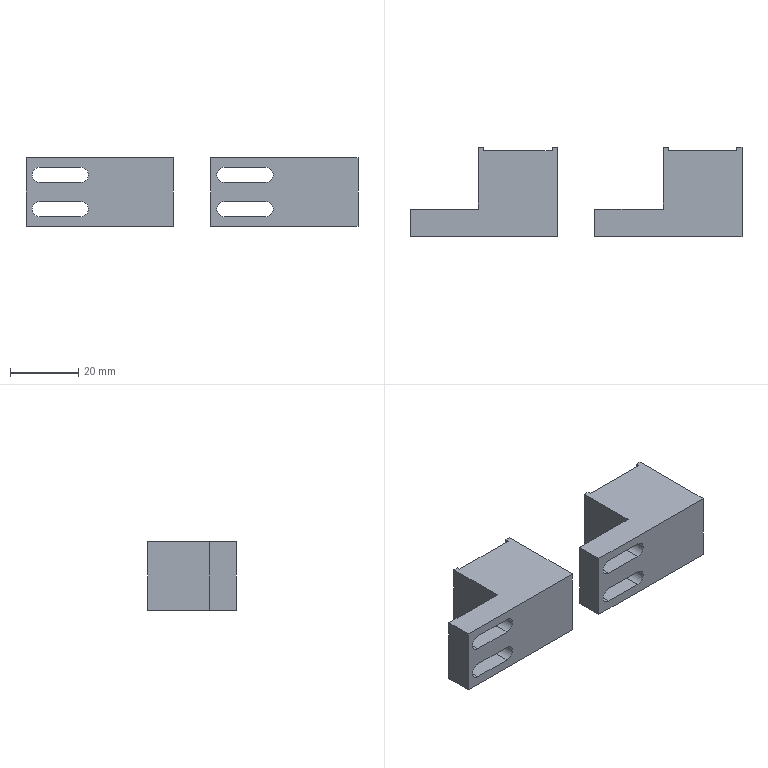Part | 2 solids | 48 faces | box 97 x 26 x 20 mm | volume 26926 mm3 | plane 32 | cylinder 12 | cone 4 | commonest cylinder face diameters 4.5 x8 3.3 x4
STEP:
#1=CARTESIAN_POINT('',(-21.5,25.,0.));
#2=VERTEX_POINT('',#1);
#3=CARTESIAN_POINT('',(-21.5,25.,20.));
#4=VERTEX_POINT('',#3);
#5=CARTESIAN_POINT('',(-21.5,25.,0.));
#6=DIRECTION('',(0.,0.,1.));
#7=VECTOR('',#6,1000.);
#8=LINE('',#5,#7);
#9=EDGE_CURVE('',#2,#4,#8,.T.);
#10=ORIENTED_EDGE('',*,*,#9,.T.);
#11=CARTESIAN_POINT('',(-1.5,25.,20.));
#12=VERTEX_POINT('',#11);
#13=CARTESIAN_POINT('',(-21.5,25.,20.));
#14=DIRECTION('',(1.,0.,0.));
#15=VECTOR('',#14,1000.);
#16=LINE('',#13,#15);
#17=EDGE_CURVE('',#4,#12,#16,.T.);
#18=ORIENTED_EDGE('',*,*,#17,.T.);
#19=CARTESIAN_POINT('',(-1.5,25.,0.));
#20=VERTEX_POINT('',#19);
#21=CARTESIAN_POINT('',(-1.5,25.,0.));
#22=DIRECTION('',(0.,0.,-1.));
#23=VECTOR('',#22,1000.);
#24=LINE('',#21,#23);
#25=EDGE_CURVE('',#12,#20,#24,.T.);
#26=ORIENTED_EDGE('',*,*,#25,.T.);
#27=CARTESIAN_POINT('',(-21.5,25.,0.));
#28=DIRECTION('',(-1.,0.,0.));
#29=VECTOR('',#28,1000.);
#30=LINE('',#27,#29);
#31=EDGE_CURVE('',#20,#2,#30,.T.);
#32=ORIENTED_EDGE('',*,*,#31,.T.);
#33=EDGE_LOOP('',(#10,#18,#26,#32));
#34=FACE_BOUND('',#33,.T.);
#35=CARTESIAN_POINT('',(-16.5,25.,11.65));
#36=VERTEX_POINT('',#35);
#37=CARTESIAN_POINT('',(-16.5,25.,10.));
#38=DIRECTION('',(0.,1.,0.));
#39=DIRECTION('',(0.,0.,1.));
#40=AXIS2_PLACEMENT_3D('',#37,#38,#39);
#41=CIRCLE('',#40,1.65);
#42=EDGE_CURVE('',#36,#36,#41,.T.);
#43=ORIENTED_EDGE('',*,*,#42,.F.);
#44=EDGE_LOOP('',(#43));
#45=FACE_BOUND('',#44,.T.);
#46=CARTESIAN_POINT('',(-6.5,25.,11.65));
#47=VERTEX_POINT('',#46);
#48=CARTESIAN_POINT('',(-6.5,25.,10.));
#49=DIRECTION('',(0.,1.,0.));
#50=DIRECTION('',(0.,0.,1.));
#51=AXIS2_PLACEMENT_3D('',#48,#49,#50);
#52=CIRCLE('',#51,1.65);
#53=EDGE_CURVE('',#47,#47,#52,.T.);
#54=ORIENTED_EDGE('',*,*,#53,.F.);
#55=EDGE_LOOP('',(#54));
#56=FACE_BOUND('',#55,.T.);
#57=CARTESIAN_POINT('',(0.,25.,0.));
#58=DIRECTION('',(0.,1.,0.));
#59=DIRECTION('',(-1.,0.,0.));
#60=AXIS2_PLACEMENT_3D('',#57,#58,#59);
#61=PLANE('',#60);
#62=ADVANCED_FACE('',(#34,#45,#56),#61,.T.);
#63=CARTESIAN_POINT('',(-1.5,26.,20.));
#64=VERTEX_POINT('',#63);
#65=CARTESIAN_POINT('',(-1.5,26.,0.));
#66=VERTEX_POINT('',#65);
#67=CARTESIAN_POINT('',(-1.5,26.,0.));
#68=DIRECTION('',(0.,0.,-1.));
#69=VECTOR('',#68,1000.);
#70=LINE('',#67,#69);
#71=EDGE_CURVE('',#64,#66,#70,.T.);
#72=ORIENTED_EDGE('',*,*,#71,.T.);
#73=CARTESIAN_POINT('',(-1.5,25.,0.));
#74=DIRECTION('',(0.,1.,0.));
#75=VECTOR('',#74,1000.);
#76=LINE('',#73,#75);
#77=EDGE_CURVE('',#20,#66,#76,.T.);
#78=ORIENTED_EDGE('',*,*,#77,.F.);
#79=ORIENTED_EDGE('',*,*,#25,.F.);
#80=CARTESIAN_POINT('',(-1.5,25.,20.));
#81=DIRECTION('',(0.,1.,0.));
#82=VECTOR('',#81,1000.);
#83=LINE('',#80,#82);
#84=EDGE_CURVE('',#12,#64,#83,.T.);
#85=ORIENTED_EDGE('',*,*,#84,.T.);
#86=EDGE_LOOP('',(#72,#78,#79,#85));
#87=FACE_BOUND('',#86,.T.);
#88=CARTESIAN_POINT('',(-1.5,25.,0.));
#89=DIRECTION('',(1.,0.,0.));
#90=DIRECTION('',(0.,0.,-1.));
#91=AXIS2_PLACEMENT_3D('',#88,#89,#90);
#92=PLANE('',#91);
#93=ADVANCED_FACE('',(#87),#92,.F.);
#94=CARTESIAN_POINT('',(-21.5,26.,0.));
#95=VERTEX_POINT('',#94);
#96=CARTESIAN_POINT('',(-21.5,26.,20.));
#97=VERTEX_POINT('',#96);
#98=CARTESIAN_POINT('',(-21.5,26.,0.));
#99=DIRECTION('',(0.,0.,1.));
#100=VECTOR('',#99,1000.);
#101=LINE('',#98,#100);
#102=EDGE_CURVE('',#95,#97,#101,.T.);
#103=ORIENTED_EDGE('',*,*,#102,.T.);
#104=CARTESIAN_POINT('',(-21.5,25.,20.));
#105=DIRECTION('',(0.,1.,0.));
#106=VECTOR('',#105,1000.);
#107=LINE('',#104,#106);
#108=EDGE_CURVE('',#4,#97,#107,.T.);
#109=ORIENTED_EDGE('',*,*,#108,.F.);
#110=ORIENTED_EDGE('',*,*,#9,.F.);
#111=CARTESIAN_POINT('',(-21.5,25.,0.));
#112=DIRECTION('',(0.,1.,0.));
#113=VECTOR('',#112,1000.);
#114=LINE('',#111,#113);
#115=EDGE_CURVE('',#2,#95,#114,.T.);
#116=ORIENTED_EDGE('',*,*,#115,.T.);
#117=EDGE_LOOP('',(#103,#109,#110,#116));
#118=FACE_BOUND('',#117,.T.);
#119=CARTESIAN_POINT('',(-21.5,25.,0.));
#120=DIRECTION('',(-1.,0.,0.));
#121=DIRECTION('',(0.,0.,1.));
#122=AXIS2_PLACEMENT_3D('',#119,#120,#121);
#123=PLANE('',#122);
#124=ADVANCED_FACE('',(#118),#123,.F.);
#125=CARTESIAN_POINT('',(-27.,0.,2.75));
#126=VERTEX_POINT('',#125);
#127=CARTESIAN_POINT('',(-27.,8.,2.75));
#128=VERTEX_POINT('',#127);
#129=CARTESIAN_POINT('',(-27.,-22.,2.75));
#130=DIRECTION('',(0.,1.,0.));
#131=VECTOR('',#130,1000.);
#132=LINE('',#129,#131);
#133=EDGE_CURVE('',#126,#128,#132,.T.);
#134=ORIENTED_EDGE('',*,*,#133,.T.);
#135=CARTESIAN_POINT('',(-39.,8.,2.75));
#136=VERTEX_POINT('',#135);
#137=CARTESIAN_POINT('',(-27.,8.,2.75));
#138=DIRECTION('',(-1.,0.,0.));
#139=VECTOR('',#138,1000.);
#140=LINE('',#137,#139);
#141=EDGE_CURVE('',#128,#136,#140,.T.);
#142=ORIENTED_EDGE('',*,*,#141,.T.);
#143=CARTESIAN_POINT('',(-39.,0.,2.75));
#144=VERTEX_POINT('',#143);
#145=CARTESIAN_POINT('',(-39.,-22.,2.75));
#146=DIRECTION('',(0.,1.,0.));
#147=VECTOR('',#146,1000.);
#148=LINE('',#145,#147);
#149=EDGE_CURVE('',#144,#136,#148,.T.);
#150=ORIENTED_EDGE('',*,*,#149,.F.);
#151=CARTESIAN_POINT('',(-43.,0.,2.75));
#152=DIRECTION('',(-1.,0.,0.));
#153=VECTOR('',#152,1000.);
#154=LINE('',#151,#153);
#155=EDGE_CURVE('',#126,#144,#154,.T.);
#156=ORIENTED_EDGE('',*,*,#155,.F.);
#157=EDGE_LOOP('',(#134,#142,#150,#156));
#158=FACE_BOUND('',#157,.T.);
#159=CARTESIAN_POINT('',(-27.,-22.,2.75));
#160=DIRECTION('',(0.,0.,-1.));
#161=DIRECTION('',(-1.,0.,0.));
#162=AXIS2_PLACEMENT_3D('',#159,#160,#161);
#163=PLANE('',#162);
#164=ADVANCED_FACE('',(#158),#163,.F.);
#165=CARTESIAN_POINT('',(-39.,0.,7.25));
#166=VERTEX_POINT('',#165);
#167=CARTESIAN_POINT('',(-39.,8.,7.25));
#168=VERTEX_POINT('',#167);
#169=CARTESIAN_POINT('',(-39.,-22.,7.25));
#170=DIRECTION('',(0.,1.,0.));
#171=VECTOR('',#170,1000.);
#172=LINE('',#169,#171);
#173=EDGE_CURVE('',#166,#168,#172,.T.);
#174=ORIENTED_EDGE('',*,*,#173,.T.);
#175=CARTESIAN_POINT('',(-27.,8.,7.25));
#176=VERTEX_POINT('',#175);
#177=CARTESIAN_POINT('',(-27.,8.,7.25));
#178=DIRECTION('',(1.,0.,0.));
#179=VECTOR('',#178,1000.);
#180=LINE('',#177,#179);
#181=EDGE_CURVE('',#168,#176,#180,.T.);
#182=ORIENTED_EDGE('',*,*,#181,.T.);
#183=CARTESIAN_POINT('',(-27.,0.,7.25));
#184=VERTEX_POINT('',#183);
#185=CARTESIAN_POINT('',(-27.,-22.,7.25));
#186=DIRECTION('',(0.,1.,0.));
#187=VECTOR('',#186,1000.);
#188=LINE('',#185,#187);
#189=EDGE_CURVE('',#184,#176,#188,.T.);
#190=ORIENTED_EDGE('',*,*,#189,.F.);
#191=CARTESIAN_POINT('',(-43.,0.,7.25));
#192=DIRECTION('',(1.,0.,0.));
#193=VECTOR('',#192,1000.);
#194=LINE('',#191,#193);
#195=EDGE_CURVE('',#166,#184,#194,.T.);
#196=ORIENTED_EDGE('',*,*,#195,.F.);
#197=EDGE_LOOP('',(#174,#182,#190,#196));
#198=FACE_BOUND('',#197,.T.);
#199=CARTESIAN_POINT('',(-27.,-22.,7.25));
#200=DIRECTION('',(0.,0.,1.));
#201=DIRECTION('',(1.,0.,0.));
#202=AXIS2_PLACEMENT_3D('',#199,#200,#201);
#203=PLANE('',#202);
#204=ADVANCED_FACE('',(#198),#203,.F.);
#205=ORIENTED_EDGE('',*,*,#189,.T.);
#206=CARTESIAN_POINT('',(-27.,8.,5.));
#207=DIRECTION('',(0.,1.,0.));
#208=DIRECTION('',(-1.,0.,0.));
#209=AXIS2_PLACEMENT_3D('',#206,#207,#208);
#210=CIRCLE('',#209,2.25);
#211=EDGE_CURVE('',#176,#128,#210,.T.);
#212=ORIENTED_EDGE('',*,*,#211,.T.);
#213=ORIENTED_EDGE('',*,*,#133,.F.);
#214=CARTESIAN_POINT('',(-27.,0.,5.));
#215=DIRECTION('',(0.,1.,0.));
#216=DIRECTION('',(0.,0.,1.));
#217=AXIS2_PLACEMENT_3D('',#214,#215,#216);
#218=CIRCLE('',#217,2.25);
#219=EDGE_CURVE('',#184,#126,#218,.T.);
#220=ORIENTED_EDGE('',*,*,#219,.F.);
#221=EDGE_LOOP('',(#205,#212,#213,#220));
#222=FACE_BOUND('',#221,.T.);
#223=CARTESIAN_POINT('',(-27.,-22.,5.));
#224=DIRECTION('',(0.,1.,0.));
#225=DIRECTION('',(-1.,0.,0.));
#226=AXIS2_PLACEMENT_3D('',#223,#224,#225);
#227=CYLINDRICAL_SURFACE('',#226,2.25);
#228=ADVANCED_FACE('',(#222),#227,.F.);
#229=CARTESIAN_POINT('',(-27.,0.,12.75));
#230=VERTEX_POINT('',#229);
#231=CARTESIAN_POINT('',(-27.,8.,12.75));
#232=VERTEX_POINT('',#231);
#233=CARTESIAN_POINT('',(-27.,-22.,12.75));
#234=DIRECTION('',(0.,1.,0.));
#235=VECTOR('',#234,1000.);
#236=LINE('',#233,#235);
#237=EDGE_CURVE('',#230,#232,#236,.T.);
#238=ORIENTED_EDGE('',*,*,#237,.T.);
#239=CARTESIAN_POINT('',(-39.,8.,12.75));
#240=VERTEX_POINT('',#239);
#241=CARTESIAN_POINT('',(-27.,8.,12.75));
#242=DIRECTION('',(-1.,0.,0.));
#243=VECTOR('',#242,1000.);
#244=LINE('',#241,#243);
#245=EDGE_CURVE('',#232,#240,#244,.T.);
#246=ORIENTED_EDGE('',*,*,#245,.T.);
#247=CARTESIAN_POINT('',(-39.,0.,12.75));
#248=VERTEX_POINT('',#247);
#249=CARTESIAN_POINT('',(-39.,-22.,12.75));
#250=DIRECTION('',(0.,1.,0.));
#251=VECTOR('',#250,1000.);
#252=LINE('',#249,#251);
#253=EDGE_CURVE('',#248,#240,#252,.T.);
#254=ORIENTED_EDGE('',*,*,#253,.F.);
#255=CARTESIAN_POINT('',(-43.,0.,12.75));
#256=DIRECTION('',(-1.,0.,0.));
#257=VECTOR('',#256,1000.);
#258=LINE('',#255,#257);
#259=EDGE_CURVE('',#230,#248,#258,.T.);
#260=ORIENTED_EDGE('',*,*,#259,.F.);
#261=EDGE_LOOP('',(#238,#246,#254,#260));
#262=FACE_BOUND('',#261,.T.);
#263=CARTESIAN_POINT('',(-27.,-22.,12.75));
#264=DIRECTION('',(0.,0.,-1.));
#265=DIRECTION('',(-1.,0.,0.));
#266=AXIS2_PLACEMENT_3D('',#263,#264,#265);
#267=PLANE('',#266);
#268=ADVANCED_FACE('',(#262),#267,.F.);
#269=CARTESIAN_POINT('',(-39.,0.,17.25));
#270=VERTEX_POINT('',#269);
#271=CARTESIAN_POINT('',(-39.,8.,17.25));
#272=VERTEX_POINT('',#271);
#273=CARTESIAN_POINT('',(-39.,-22.,17.25));
#274=DIRECTION('',(0.,1.,0.));
#275=VECTOR('',#274,1000.);
#276=LINE('',#273,#275);
#277=EDGE_CURVE('',#270,#272,#276,.T.);
#278=ORIENTED_EDGE('',*,*,#277,.T.);
#279=CARTESIAN_POINT('',(-27.,8.,17.25));
#280=VERTEX_POINT('',#279);
#281=CARTESIAN_POINT('',(-27.,8.,17.25));
#282=DIRECTION('',(1.,0.,0.));
#283=VECTOR('',#282,1000.);
#284=LINE('',#281,#283);
#285=EDGE_CURVE('',#272,#280,#284,.T.);
#286=ORIENTED_EDGE('',*,*,#285,.T.);
#287=CARTESIAN_POINT('',(-27.,0.,17.25));
#288=VERTEX_POINT('',#287);
#289=CARTESIAN_POINT('',(-27.,-22.,17.25));
#290=DIRECTION('',(0.,1.,0.));
#291=VECTOR('',#290,1000.);
#292=LINE('',#289,#291);
#293=EDGE_CURVE('',#288,#280,#292,.T.);
#294=ORIENTED_EDGE('',*,*,#293,.F.);
#295=CARTESIAN_POINT('',(-43.,0.,17.25));
#296=DIRECTION('',(1.,0.,0.));
#297=VECTOR('',#296,1000.);
#298=LINE('',#295,#297);
#299=EDGE_CURVE('',#270,#288,#298,.T.);
#300=ORIENTED_EDGE('',*,*,#299,.F.);
#301=EDGE_LOOP('',(#278,#286,#294,#300));
#302=FACE_BOUND('',#301,.T.);
#303=CARTESIAN_POINT('',(-27.,-22.,17.25));
#304=DIRECTION('',(0.,0.,1.));
#305=DIRECTION('',(1.,0.,0.));
#306=AXIS2_PLACEMENT_3D('',#303,#304,#305);
#307=PLANE('',#306);
#308=ADVANCED_FACE('',(#302),#307,.F.);
#309=ORIENTED_EDGE('',*,*,#293,.T.);
#310=CARTESIAN_POINT('',(-27.,8.,15.));
#311=DIRECTION('',(0.,1.,0.));
#312=DIRECTION('',(1.,0.,0.));
#313=AXIS2_PLACEMENT_3D('',#310,#311,#312);
#314=CIRCLE('',#313,2.25);
#315=EDGE_CURVE('',#280,#232,#314,.T.);
#316=ORIENTED_EDGE('',*,*,#315,.T.);
#317=ORIENTED_EDGE('',*,*,#237,.F.);
#318=CARTESIAN_POINT('',(-27.,0.,15.));
#319=DIRECTION('',(0.,1.,0.));
#320=DIRECTION('',(0.,0.,1.));
#321=AXIS2_PLACEMENT_3D('',#318,#319,#320);
#322=CIRCLE('',#321,2.25);
#323=EDGE_CURVE('',#288,#230,#322,.T.);
#324=ORIENTED_EDGE('',*,*,#323,.F.);
#325=EDGE_LOOP('',(#309,#316,#317,#324));
#326=FACE_BOUND('',#325,.T.);
#327=CARTESIAN_POINT('',(-27.,-22.,15.));
#328=DIRECTION('',(0.,1.,0.));
#329=DIRECTION('',(-1.,0.,0.));
#330=AXIS2_PLACEMENT_3D('',#327,#328,#329);
#331=CYLINDRICAL_SURFACE('',#330,2.25);
#332=ADVANCED_FACE('',(#326),#331,.F.);
#333=CARTESIAN_POINT('',(-23.,26.,0.));
#334=VERTEX_POINT('',#333);
#335=CARTESIAN_POINT('',(0.,26.,0.));
#336=DIRECTION('',(-1.,0.,0.));
#337=VECTOR('',#336,1000.);
#338=LINE('',#335,#337);
#339=EDGE_CURVE('',#95,#334,#338,.T.);
#340=ORIENTED_EDGE('',*,*,#339,.F.);
#341=ORIENTED_EDGE('',*,*,#115,.F.);
#342=ORIENTED_EDGE('',*,*,#31,.F.);
#343=ORIENTED_EDGE('',*,*,#77,.T.);
#344=CARTESIAN_POINT('',(0.,26.,0.));
#345=VERTEX_POINT('',#344);
#346=CARTESIAN_POINT('',(0.,26.,0.));
#347=DIRECTION('',(-1.,0.,0.));
#348=VECTOR('',#347,1000.);
#349=LINE('',#346,#348);
#350=EDGE_CURVE('',#345,#66,#349,.T.);
#351=ORIENTED_EDGE('',*,*,#350,.F.);
#352=CARTESIAN_POINT('',(0.,0.,0.));
#353=VERTEX_POINT('',#352);
#354=CARTESIAN_POINT('',(0.,0.,0.));
#355=DIRECTION('',(0.,1.,0.));
#356=VECTOR('',#355,1000.);
#357=LINE('',#354,#356);
#358=EDGE_CURVE('',#353,#345,#357,.T.);
#359=ORIENTED_EDGE('',*,*,#358,.F.);
#360=CARTESIAN_POINT('',(-43.,0.,0.));
#361=VERTEX_POINT('',#360);
#362=CARTESIAN_POINT('',(-43.,0.,0.));
#363=DIRECTION('',(1.,0.,0.));
#364=VECTOR('',#363,1000.);
#365=LINE('',#362,#364);
#366=EDGE_CURVE('',#361,#353,#365,.T.);
#367=ORIENTED_EDGE('',*,*,#366,.F.);
#368=CARTESIAN_POINT('',(-43.,8.,0.));
#369=VERTEX_POINT('',#368);
#370=CARTESIAN_POINT('',(-43.,8.,0.));
#371=DIRECTION('',(0.,-1.,0.));
#372=VECTOR('',#371,1000.);
#373=LINE('',#370,#372);
#374=EDGE_CURVE('',#369,#361,#373,.T.);
#375=ORIENTED_EDGE('',*,*,#374,.F.);
#376=CARTESIAN_POINT('',(-23.,8.,0.));
#377=VERTEX_POINT('',#376);
#378=CARTESIAN_POINT('',(-23.,8.,0.));
#379=DIRECTION('',(-1.,0.,0.));
#380=VECTOR('',#379,1000.);
#381=LINE('',#378,#380);
#382=EDGE_CURVE('',#377,#369,#381,.T.);
#383=ORIENTED_EDGE('',*,*,#382,.F.);
#384=CARTESIAN_POINT('',(-23.,26.,0.));
#385=DIRECTION('',(0.,-1.,0.));
#386=VECTOR('',#385,1000.);
#387=LINE('',#384,#386);
#388=EDGE_CURVE('',#334,#377,#387,.T.);
#389=ORIENTED_EDGE('',*,*,#388,.F.);
#390=EDGE_LOOP('',(#340,#341,#342,#343,#351,#359,#367,#375,#383,#389));
#391=FACE_BOUND('',#390,.T.);
#392=CARTESIAN_POINT('',(0.,0.,0.));
#393=DIRECTION('',(0.,0.,1.));
#394=DIRECTION('',(1.,0.,0.));
#395=AXIS2_PLACEMENT_3D('',#392,#393,#394);
#396=PLANE('',#395);
#397=ADVANCED_FACE('',(#391),#396,.F.);
#398=ORIENTED_EDGE('',*,*,#108,.T.);
#399=CARTESIAN_POINT('',(-23.,26.,20.));
#400=VERTEX_POINT('',#399);
#401=CARTESIAN_POINT('',(0.,26.,20.));
#402=DIRECTION('',(-1.,0.,0.));
#403=VECTOR('',#402,1000.);
#404=LINE('',#401,#403);
#405=EDGE_CURVE('',#97,#400,#404,.T.);
#406=ORIENTED_EDGE('',*,*,#405,.T.);
#407=CARTESIAN_POINT('',(-23.,8.,20.));
#408=VERTEX_POINT('',#407);
#409=CARTESIAN_POINT('',(-23.,26.,20.));
#410=DIRECTION('',(0.,-1.,0.));
#411=VECTOR('',#410,1000.);
#412=LINE('',#409,#411);
#413=EDGE_CURVE('',#400,#408,#412,.T.);
#414=ORIENTED_EDGE('',*,*,#413,.T.);
#415=CARTESIAN_POINT('',(-43.,8.,20.));
#416=VERTEX_POINT('',#415);
#417=CARTESIAN_POINT('',(-23.,8.,20.));
#418=DIRECTION('',(-1.,0.,0.));
#419=VECTOR('',#418,1000.);
#420=LINE('',#417,#419);
#421=EDGE_CURVE('',#408,#416,#420,.T.);
#422=ORIENTED_EDGE('',*,*,#421,.T.);
#423=CARTESIAN_POINT('',(-43.,0.,20.));
#424=VERTEX_POINT('',#423);
#425=CARTESIAN_POINT('',(-43.,8.,20.));
#426=DIRECTION('',(0.,-1.,0.));
#427=VECTOR('',#426,1000.);
#428=LINE('',#425,#427);
#429=EDGE_CURVE('',#416,#424,#428,.T.);
#430=ORIENTED_EDGE('',*,*,#429,.T.);
#431=CARTESIAN_POINT('',(0.,0.,20.));
#432=VERTEX_POINT('',#431);
#433=CARTESIAN_POINT('',(-43.,0.,20.));
#434=DIRECTION('',(1.,0.,0.));
#435=VECTOR('',#434,1000.);
#436=LINE('',#433,#435);
#437=EDGE_CURVE('',#424,#432,#436,.T.);
#438=ORIENTED_EDGE('',*,*,#437,.T.);
#439=CARTESIAN_POINT('',(0.,26.,20.));
#440=VERTEX_POINT('',#439);
#441=CARTESIAN_POINT('',(0.,0.,20.));
#442=DIRECTION('',(0.,1.,0.));
#443=VECTOR('',#442,1000.);
#444=LINE('',#441,#443);
#445=EDGE_CURVE('',#432,#440,#444,.T.);
#446=ORIENTED_EDGE('',*,*,#445,.T.);
#447=CARTESIAN_POINT('',(0.,26.,20.));
#448=DIRECTION('',(-1.,0.,0.));
#449=VECTOR('',#448,1000.);
#450=LINE('',#447,#449);
#451=EDGE_CURVE('',#440,#64,#450,.T.);
#452=ORIENTED_EDGE('',*,*,#451,.T.);
#453=ORIENTED_EDGE('',*,*,#84,.F.);
#454=ORIENTED_EDGE('',*,*,#17,.F.);
#455=EDGE_LOOP('',(#398,#406,#414,#422,#430,#438,#446,#452,#453,#454));
#456=FACE_BOUND('',#455,.T.);
#457=CARTESIAN_POINT('',(0.,0.,20.));
#458=DIRECTION('',(0.,0.,1.));
#459=DIRECTION('',(1.,0.,0.));
#460=AXIS2_PLACEMENT_3D('',#457,#458,#459);
#461=PLANE('',#460);
#462=ADVANCED_FACE('',(#456),#461,.T.);
#463=ORIENTED_EDGE('',*,*,#374,.T.);
#464=CARTESIAN_POINT('',(-43.,0.,20.));
#465=DIRECTION('',(0.,0.,-1.));
#466=VECTOR('',#465,1000.);
#467=LINE('',#464,#466);
#468=EDGE_CURVE('',#424,#361,#467,.T.);
#469=ORIENTED_EDGE('',*,*,#468,.F.);
#470=ORIENTED_EDGE('',*,*,#429,.F.);
#471=CARTESIAN_POINT('',(-43.,8.,20.));
#472=DIRECTION('',(0.,0.,-1.));
#473=VECTOR('',#472,1000.);
#474=LINE('',#471,#473);
#475=EDGE_CURVE('',#416,#369,#474,.T.);
#476=ORIENTED_EDGE('',*,*,#475,.T.);
#477=EDGE_LOOP('',(#463,#469,#470,#476));
#478=FACE_BOUND('',#477,.T.);
#479=CARTESIAN_POINT('',(-43.,8.,20.));
#480=DIRECTION('',(1.,0.,0.));
#481=DIRECTION('',(0.,1.,0.));
#482=AXIS2_PLACEMENT_3D('',#479,#480,#481);
#483=PLANE('',#482);
#484=ADVANCED_FACE('',(#478),#483,.F.);
#485=ORIENTED_EDGE('',*,*,#382,.T.);
#486=ORIENTED_EDGE('',*,*,#475,.F.);
#487=ORIENTED_EDGE('',*,*,#421,.F.);
#488=CARTESIAN_POINT('',(-23.,8.,20.));
#489=DIRECTION('',(0.,0.,-1.));
#490=VECTOR('',#489,1000.);
#491=LINE('',#488,#490);
#492=EDGE_CURVE('',#408,#377,#491,.T.);
#493=ORIENTED_EDGE('',*,*,#492,.T.);
#494=EDGE_LOOP('',(#485,#486,#487,#493));
#495=FACE_BOUND('',#494,.T.);
#496=ORIENTED_EDGE('',*,*,#245,.F.);
#497=ORIENTED_EDGE('',*,*,#315,.F.);
#498=ORIENTED_EDGE('',*,*,#285,.F.);
#499=CARTESIAN_POINT('',(-39.,8.,15.));
#500=DIRECTION('',(0.,1.,0.));
#501=DIRECTION('',(1.,0.,0.));
#502=AXIS2_PLACEMENT_3D('',#499,#500,#501);
#503=CIRCLE('',#502,2.25);
#504=EDGE_CURVE('',#240,#272,#503,.T.);
#505=ORIENTED_EDGE('',*,*,#504,.F.);
#506=EDGE_LOOP('',(#496,#497,#498,#505));
#507=FACE_BOUND('',#506,.T.);
#508=ORIENTED_EDGE('',*,*,#141,.F.);
#509=ORIENTED_EDGE('',*,*,#211,.F.);
#510=ORIENTED_EDGE('',*,*,#181,.F.);
#511=CARTESIAN_POINT('',(-39.,8.,5.));
#512=DIRECTION('',(0.,1.,0.));
#513=DIRECTION('',(-1.,0.,0.));
#514=AXIS2_PLACEMENT_3D('',#511,#512,#513);
#515=CIRCLE('',#514,2.25);
#516=EDGE_CURVE('',#136,#168,#515,.T.);
#517=ORIENTED_EDGE('',*,*,#516,.F.);
#518=EDGE_LOOP('',(#508,#509,#510,#517));
#519=FACE_BOUND('',#518,.T.);
#520=CARTESIAN_POINT('',(-23.,8.,20.));
#521=DIRECTION('',(0.,-1.,0.));
#522=DIRECTION('',(0.,0.,-1.));
#523=AXIS2_PLACEMENT_3D('',#520,#521,#522);
#524=PLANE('',#523);
#525=ADVANCED_FACE('',(#495,#507,#519),#524,.F.);
#526=ORIENTED_EDGE('',*,*,#388,.T.);
#527=ORIENTED_EDGE('',*,*,#492,.F.);
#528=ORIENTED_EDGE('',*,*,#413,.F.);
#529=CARTESIAN_POINT('',(-23.,26.,20.));
#530=DIRECTION('',(0.,0.,-1.));
#531=VECTOR('',#530,1000.);
#532=LINE('',#529,#531);
#533=EDGE_CURVE('',#400,#334,#532,.T.);
#534=ORIENTED_EDGE('',*,*,#533,.T.);
#535=EDGE_LOOP('',(#526,#527,#528,#534));
#536=FACE_BOUND('',#535,.T.);
#537=CARTESIAN_POINT('',(-23.,26.,20.));
#538=DIRECTION('',(1.,0.,0.));
#539=DIRECTION('',(0.,1.,0.));
#540=AXIS2_PLACEMENT_3D('',#537,#538,#539);
#541=PLANE('',#540);
#542=ADVANCED_FACE('',(#536),#541,.F.);
#543=ORIENTED_EDGE('',*,*,#350,.T.);
#544=ORIENTED_EDGE('',*,*,#71,.F.);
#545=ORIENTED_EDGE('',*,*,#451,.F.);
#546=CARTESIAN_POINT('',(0.,26.,20.));
#547=DIRECTION('',(0.,0.,-1.));
#548=VECTOR('',#547,1000.);
#549=LINE('',#546,#548);
#550=EDGE_CURVE('',#440,#345,#549,.T.);
#551=ORIENTED_EDGE('',*,*,#550,.T.);
#552=EDGE_LOOP('',(#543,#544,#545,#551));
#553=FACE_BOUND('',#552,.T.);
#554=CARTESIAN_POINT('',(0.,26.,20.));
#555=DIRECTION('',(0.,-1.,0.));
#556=DIRECTION('',(1.,0.,0.));
#557=AXIS2_PLACEMENT_3D('',#554,#555,#556);
#558=PLANE('',#557);
#559=ADVANCED_FACE('',(#553),#558,.F.);
#560=ORIENTED_EDGE('',*,*,#358,.T.);
#561=ORIENTED_EDGE('',*,*,#550,.F.);
#562=ORIENTED_EDGE('',*,*,#445,.F.);
#563=CARTESIAN_POINT('',(0.,0.,20.));
#564=DIRECTION('',(0.,0.,-1.));
#565=VECTOR('',#564,1000.);
#566=LINE('',#563,#565);
#567=EDGE_CURVE('',#432,#353,#566,.T.);
#568=ORIENTED_EDGE('',*,*,#567,.T.);
#569=EDGE_LOOP('',(#560,#561,#562,#568));
#570=FACE_BOUND('',#569,.T.);
#571=CARTESIAN_POINT('',(0.,0.,20.));
#572=DIRECTION('',(-1.,0.,0.));
#573=DIRECTION('',(0.,0.,1.));
#574=AXIS2_PLACEMENT_3D('',#571,#572,#573);
#575=PLANE('',#574);
#576=ADVANCED_FACE('',(#570),#575,.F.);
#577=ORIENTED_EDGE('',*,*,#366,.T.);
#578=ORIENTED_EDGE('',*,*,#567,.F.);
#579=ORIENTED_EDGE('',*,*,#437,.F.);
#580=ORIENTED_EDGE('',*,*,#468,.T.);
#581=EDGE_LOOP('',(#577,#578,#579,#580));
#582=FACE_BOUND('',#581,.T.);
#583=ORIENTED_EDGE('',*,*,#299,.T.);
#584=ORIENTED_EDGE('',*,*,#323,.T.);
#585=ORIENTED_EDGE('',*,*,#259,.T.);
#586=CARTESIAN_POINT('',(-39.,0.,15.));
#587=DIRECTION('',(0.,1.,0.));
#588=DIRECTION('',(0.,0.,1.));
#589=AXIS2_PLACEMENT_3D('',#586,#587,#588);
#590=CIRCLE('',#589,2.25);
#591=EDGE_CURVE('',#248,#270,#590,.T.);
#592=ORIENTED_EDGE('',*,*,#591,.T.);
#593=EDGE_LOOP('',(#583,#584,#585,#592));
#594=FACE_BOUND('',#593,.T.);
#595=ORIENTED_EDGE('',*,*,#195,.T.);
#596=ORIENTED_EDGE('',*,*,#219,.T.);
#597=ORIENTED_EDGE('',*,*,#155,.T.);
#598=CARTESIAN_POINT('',(-39.,0.,5.));
#599=DIRECTION('',(0.,1.,0.));
#600=DIRECTION('',(0.,0.,1.));
#601=AXIS2_PLACEMENT_3D('',#598,#599,#600);
#602=CIRCLE('',#601,2.25);
#603=EDGE_CURVE('',#144,#166,#602,.T.);
#604=ORIENTED_EDGE('',*,*,#603,.T.);
#605=EDGE_LOOP('',(#595,#596,#597,#604));
#606=FACE_BOUND('',#605,.T.);
#607=CARTESIAN_POINT('',(-43.,0.,20.));
#608=DIRECTION('',(0.,1.,0.));
#609=DIRECTION('',(0.,0.,1.));
#610=AXIS2_PLACEMENT_3D('',#607,#608,#609);
#611=PLANE('',#610);
#612=ADVANCED_FACE('',(#582,#594,#606),#611,.F.);
#613=ORIENTED_EDGE('',*,*,#405,.F.);
#614=ORIENTED_EDGE('',*,*,#102,.F.);
#615=ORIENTED_EDGE('',*,*,#339,.T.);
#616=ORIENTED_EDGE('',*,*,#533,.F.);
#617=EDGE_LOOP('',(#613,#614,#615,#616));
#618=FACE_BOUND('',#617,.T.);
#619=CARTESIAN_POINT('',(0.,26.,20.));
#620=DIRECTION('',(0.,-1.,0.));
#621=DIRECTION('',(1.,0.,0.));
#622=AXIS2_PLACEMENT_3D('',#619,#620,#621);
#623=PLANE('',#622);
#624=ADVANCED_FACE('',(#618),#623,.F.);
#625=ORIENTED_EDGE('',*,*,#591,.F.);
#626=ORIENTED_EDGE('',*,*,#253,.T.);
#627=ORIENTED_EDGE('',*,*,#504,.T.);
#628=ORIENTED_EDGE('',*,*,#277,.F.);
#629=EDGE_LOOP('',(#625,#626,#627,#628));
#630=FACE_BOUND('',#629,.T.);
#631=CARTESIAN_POINT('',(-39.,-22.,15.));
#632=DIRECTION('',(0.,1.,0.));
#633=DIRECTION('',(-1.,0.,0.));
#634=AXIS2_PLACEMENT_3D('',#631,#632,#633);
#635=CYLINDRICAL_SURFACE('',#634,2.25);
#636=ADVANCED_FACE('',(#630),#635,.F.);
#637=ORIENTED_EDGE('',*,*,#603,.F.);
#638=ORIENTED_EDGE('',*,*,#149,.T.);
#639=ORIENTED_EDGE('',*,*,#516,.T.);
#640=ORIENTED_EDGE('',*,*,#173,.F.);
#641=EDGE_LOOP('',(#637,#638,#639,#640));
#642=FACE_BOUND('',#641,.T.);
#643=CARTESIAN_POINT('',(-39.,-22.,5.));
#644=DIRECTION('',(0.,1.,0.));
#645=DIRECTION('',(-1.,0.,0.));
#646=AXIS2_PLACEMENT_3D('',#643,#644,#645);
#647=CYLINDRICAL_SURFACE('',#646,2.25);
#648=ADVANCED_FACE('',(#642),#647,.F.);
#649=CARTESIAN_POINT('',(-16.5,14.9,11.65));
#650=VERTEX_POINT('',#649);
#651=CARTESIAN_POINT('',(-16.5,14.9,10.));
#652=DIRECTION('',(0.,1.,0.));
#653=DIRECTION('',(0.,0.,1.));
#654=AXIS2_PLACEMENT_3D('',#651,#652,#653);
#655=CIRCLE('',#654,1.65);
#656=EDGE_CURVE('',#650,#650,#655,.T.);
#657=ORIENTED_EDGE('',*,*,#656,.T.);
#658=EDGE_LOOP('',(#657));
#659=FACE_BOUND('',#658,.T.);
#660=CARTESIAN_POINT('',(-16.5,13.909,10.));
#661=VERTEX_POINT('',#660);
#662=VERTEX_LOOP('',#661);
#663=FACE_BOUND('',#662,.T.);
#664=CARTESIAN_POINT('',(-16.5,14.9,10.));
#665=DIRECTION('',(0.,1.,0.));
#666=DIRECTION('',(0.,0.,1.));
#667=AXIS2_PLACEMENT_3D('',#664,#665,#666);
#668=CONICAL_SURFACE('',#667,1.65,1.03);
#669=ADVANCED_FACE('',(#659,#663),#668,.F.);
#670=ORIENTED_EDGE('',*,*,#656,.F.);
#671=EDGE_LOOP('',(#670));
#672=FACE_BOUND('',#671,.T.);
#673=ORIENTED_EDGE('',*,*,#42,.T.);
#674=EDGE_LOOP('',(#673));
#675=FACE_BOUND('',#674,.T.);
#676=CARTESIAN_POINT('',(-16.5,25.,10.));
#677=DIRECTION('',(0.,1.,0.));
#678=DIRECTION('',(0.,0.,1.));
#679=AXIS2_PLACEMENT_3D('',#676,#677,#678);
#680=CYLINDRICAL_SURFACE('',#679,1.65);
#681=ADVANCED_FACE('',(#672,#675),#680,.F.);
#682=CARTESIAN_POINT('',(-6.5,14.9,11.65));
#683=VERTEX_POINT('',#682);
#684=CARTESIAN_POINT('',(-6.5,14.9,10.));
#685=DIRECTION('',(0.,1.,0.));
#686=DIRECTION('',(0.,0.,1.));
#687=AXIS2_PLACEMENT_3D('',#684,#685,#686);
#688=CIRCLE('',#687,1.65);
#689=EDGE_CURVE('',#683,#683,#688,.T.);
#690=ORIENTED_EDGE('',*,*,#689,.T.);
#691=EDGE_LOOP('',(#690));
#692=FACE_BOUND('',#691,.T.);
#693=CARTESIAN_POINT('',(-6.5,13.909,10.));
#694=VERTEX_POINT('',#693);
#695=VERTEX_LOOP('',#694);
#696=FACE_BOUND('',#695,.T.);
#697=CARTESIAN_POINT('',(-6.5,14.9,10.));
#698=DIRECTION('',(0.,1.,0.));
#699=DIRECTION('',(0.,0.,1.));
#700=AXIS2_PLACEMENT_3D('',#697,#698,#699);
#701=CONICAL_SURFACE('',#700,1.65,1.03);
#702=ADVANCED_FACE('',(#692,#696),#701,.F.);
#703=ORIENTED_EDGE('',*,*,#689,.F.);
#704=EDGE_LOOP('',(#703));
#705=FACE_BOUND('',#704,.T.);
#706=ORIENTED_EDGE('',*,*,#53,.T.);
#707=EDGE_LOOP('',(#706));
#708=FACE_BOUND('',#707,.T.);
#709=CARTESIAN_POINT('',(-6.5,25.,10.));
#710=DIRECTION('',(0.,1.,0.));
#711=DIRECTION('',(0.,0.,1.));
#712=AXIS2_PLACEMENT_3D('',#709,#710,#711);
#713=CYLINDRICAL_SURFACE('',#712,1.65);
#714=ADVANCED_FACE('',(#705,#708),#713,.F.);
#715=CLOSED_SHELL('',(#62,#93,#124,#164,#204,#228,#268,#308,#332,#397,#462,#484,#525,#542,#559,#576,#612,#624,#636,#648,#669,#681,#702,#714));
#716=MANIFOLD_SOLID_BREP('',#715);
#717=CARTESIAN_POINT('',(32.5,25.,0.));
#718=VERTEX_POINT('',#717);
#719=CARTESIAN_POINT('',(32.5,25.,20.));
#720=VERTEX_POINT('',#719);
#721=CARTESIAN_POINT('',(32.5,25.,0.));
#722=DIRECTION('',(0.,0.,1.));
#723=VECTOR('',#722,1000.);
#724=LINE('',#721,#723);
#725=EDGE_CURVE('',#718,#720,#724,.T.);
#726=ORIENTED_EDGE('',*,*,#725,.T.);
#727=CARTESIAN_POINT('',(52.5,25.,20.));
#728=VERTEX_POINT('',#727);
#729=CARTESIAN_POINT('',(32.5,25.,20.));
#730=DIRECTION('',(1.,0.,0.));
#731=VECTOR('',#730,1000.);
#732=LINE('',#729,#731);
#733=EDGE_CURVE('',#720,#728,#732,.T.);
#734=ORIENTED_EDGE('',*,*,#733,.T.);
#735=CARTESIAN_POINT('',(52.5,25.,0.));
#736=VERTEX_POINT('',#735);
#737=CARTESIAN_POINT('',(52.5,25.,0.));
#738=DIRECTION('',(0.,0.,-1.));
#739=VECTOR('',#738,1000.);
#740=LINE('',#737,#739);
#741=EDGE_CURVE('',#728,#736,#740,.T.);
#742=ORIENTED_EDGE('',*,*,#741,.T.);
#743=CARTESIAN_POINT('',(32.5,25.,0.));
#744=DIRECTION('',(-1.,0.,0.));
#745=VECTOR('',#744,1000.);
#746=LINE('',#743,#745);
#747=EDGE_CURVE('',#736,#718,#746,.T.);
#748=ORIENTED_EDGE('',*,*,#747,.T.);
#749=EDGE_LOOP('',(#726,#734,#742,#748));
#750=FACE_BOUND('',#749,.T.);
#751=CARTESIAN_POINT('',(37.5,25.,11.65));
#752=VERTEX_POINT('',#751);
#753=CARTESIAN_POINT('',(37.5,25.,10.));
#754=DIRECTION('',(0.,1.,0.));
#755=DIRECTION('',(0.,0.,1.));
#756=AXIS2_PLACEMENT_3D('',#753,#754,#755);
#757=CIRCLE('',#756,1.65);
#758=EDGE_CURVE('',#752,#752,#757,.T.);
#759=ORIENTED_EDGE('',*,*,#758,.F.);
#760=EDGE_LOOP('',(#759));
#761=FACE_BOUND('',#760,.T.);
#762=CARTESIAN_POINT('',(47.5,25.,11.65));
#763=VERTEX_POINT('',#762);
#764=CARTESIAN_POINT('',(47.5,25.,10.));
#765=DIRECTION('',(0.,1.,0.));
#766=DIRECTION('',(0.,0.,1.));
#767=AXIS2_PLACEMENT_3D('',#764,#765,#766);
#768=CIRCLE('',#767,1.65);
#769=EDGE_CURVE('',#763,#763,#768,.T.);
#770=ORIENTED_EDGE('',*,*,#769,.F.);
#771=EDGE_LOOP('',(#770));
#772=FACE_BOUND('',#771,.T.);
#773=CARTESIAN_POINT('',(54.,25.,0.));
#774=DIRECTION('',(0.,1.,0.));
#775=DIRECTION('',(-1.,0.,0.));
#776=AXIS2_PLACEMENT_3D('',#773,#774,#775);
#777=PLANE('',#776);
#778=ADVANCED_FACE('',(#750,#761,#772),#777,.T.);
#779=CARTESIAN_POINT('',(52.5,26.,20.));
#780=VERTEX_POINT('',#779);
#781=CARTESIAN_POINT('',(52.5,26.,0.));
#782=VERTEX_POINT('',#781);
#783=CARTESIAN_POINT('',(52.5,26.,0.));
#784=DIRECTION('',(0.,0.,-1.));
#785=VECTOR('',#784,1000.);
#786=LINE('',#783,#785);
#787=EDGE_CURVE('',#780,#782,#786,.T.);
#788=ORIENTED_EDGE('',*,*,#787,.T.);
#789=CARTESIAN_POINT('',(52.5,25.,0.));
#790=DIRECTION('',(0.,1.,0.));
#791=VECTOR('',#790,1000.);
#792=LINE('',#789,#791);
#793=EDGE_CURVE('',#736,#782,#792,.T.);
#794=ORIENTED_EDGE('',*,*,#793,.F.);
#795=ORIENTED_EDGE('',*,*,#741,.F.);
#796=CARTESIAN_POINT('',(52.5,25.,20.));
#797=DIRECTION('',(0.,1.,0.));
#798=VECTOR('',#797,1000.);
#799=LINE('',#796,#798);
#800=EDGE_CURVE('',#728,#780,#799,.T.);
#801=ORIENTED_EDGE('',*,*,#800,.T.);
#802=EDGE_LOOP('',(#788,#794,#795,#801));
#803=FACE_BOUND('',#802,.T.);
#804=CARTESIAN_POINT('',(52.5,25.,0.));
#805=DIRECTION('',(1.,0.,0.));
#806=DIRECTION('',(0.,0.,-1.));
#807=AXIS2_PLACEMENT_3D('',#804,#805,#806);
#808=PLANE('',#807);
#809=ADVANCED_FACE('',(#803),#808,.F.);
#810=CARTESIAN_POINT('',(32.5,26.,0.));
#811=VERTEX_POINT('',#810);
#812=CARTESIAN_POINT('',(32.5,26.,20.));
#813=VERTEX_POINT('',#812);
#814=CARTESIAN_POINT('',(32.5,26.,0.));
#815=DIRECTION('',(0.,0.,1.));
#816=VECTOR('',#815,1000.);
#817=LINE('',#814,#816);
#818=EDGE_CURVE('',#811,#813,#817,.T.);
#819=ORIENTED_EDGE('',*,*,#818,.T.);
#820=CARTESIAN_POINT('',(32.5,25.,20.));
#821=DIRECTION('',(0.,1.,0.));
#822=VECTOR('',#821,1000.);
#823=LINE('',#820,#822);
#824=EDGE_CURVE('',#720,#813,#823,.T.);
#825=ORIENTED_EDGE('',*,*,#824,.F.);
#826=ORIENTED_EDGE('',*,*,#725,.F.);
#827=CARTESIAN_POINT('',(32.5,25.,0.));
#828=DIRECTION('',(0.,1.,0.));
#829=VECTOR('',#828,1000.);
#830=LINE('',#827,#829);
#831=EDGE_CURVE('',#718,#811,#830,.T.);
#832=ORIENTED_EDGE('',*,*,#831,.T.);
#833=EDGE_LOOP('',(#819,#825,#826,#832));
#834=FACE_BOUND('',#833,.T.);
#835=CARTESIAN_POINT('',(32.5,25.,0.));
#836=DIRECTION('',(-1.,0.,0.));
#837=DIRECTION('',(0.,0.,1.));
#838=AXIS2_PLACEMENT_3D('',#835,#836,#837);
#839=PLANE('',#838);
#840=ADVANCED_FACE('',(#834),#839,.F.);
#841=CARTESIAN_POINT('',(27.,0.,2.75));
#842=VERTEX_POINT('',#841);
#843=CARTESIAN_POINT('',(27.,8.,2.75));
#844=VERTEX_POINT('',#843);
#845=CARTESIAN_POINT('',(27.,-22.,2.75));
#846=DIRECTION('',(0.,1.,0.));
#847=VECTOR('',#846,1000.);
#848=LINE('',#845,#847);
#849=EDGE_CURVE('',#842,#844,#848,.T.);
#850=ORIENTED_EDGE('',*,*,#849,.T.);
#851=CARTESIAN_POINT('',(15.,8.,2.75));
#852=VERTEX_POINT('',#851);
#853=CARTESIAN_POINT('',(27.,8.,2.75));
#854=DIRECTION('',(-1.,0.,0.));
#855=VECTOR('',#854,1000.);
#856=LINE('',#853,#855);
#857=EDGE_CURVE('',#844,#852,#856,.T.);
#858=ORIENTED_EDGE('',*,*,#857,.T.);
#859=CARTESIAN_POINT('',(15.,0.,2.75));
#860=VERTEX_POINT('',#859);
#861=CARTESIAN_POINT('',(15.,-22.,2.75));
#862=DIRECTION('',(0.,1.,0.));
#863=VECTOR('',#862,1000.);
#864=LINE('',#861,#863);
#865=EDGE_CURVE('',#860,#852,#864,.T.);
#866=ORIENTED_EDGE('',*,*,#865,.F.);
#867=CARTESIAN_POINT('',(11.,0.,2.75));
#868=DIRECTION('',(-1.,0.,0.));
#869=VECTOR('',#868,1000.);
#870=LINE('',#867,#869);
#871=EDGE_CURVE('',#842,#860,#870,.T.);
#872=ORIENTED_EDGE('',*,*,#871,.F.);
#873=EDGE_LOOP('',(#850,#858,#866,#872));
#874=FACE_BOUND('',#873,.T.);
#875=CARTESIAN_POINT('',(27.,-22.,2.75));
#876=DIRECTION('',(0.,0.,-1.));
#877=DIRECTION('',(-1.,0.,0.));
#878=AXIS2_PLACEMENT_3D('',#875,#876,#877);
#879=PLANE('',#878);
#880=ADVANCED_FACE('',(#874),#879,.F.);
#881=CARTESIAN_POINT('',(15.,0.,7.25));
#882=VERTEX_POINT('',#881);
#883=CARTESIAN_POINT('',(15.,8.,7.25));
#884=VERTEX_POINT('',#883);
#885=CARTESIAN_POINT('',(15.,-22.,7.25));
#886=DIRECTION('',(0.,1.,0.));
#887=VECTOR('',#886,1000.);
#888=LINE('',#885,#887);
#889=EDGE_CURVE('',#882,#884,#888,.T.);
#890=ORIENTED_EDGE('',*,*,#889,.T.);
#891=CARTESIAN_POINT('',(27.,8.,7.25));
#892=VERTEX_POINT('',#891);
#893=CARTESIAN_POINT('',(27.,8.,7.25));
#894=DIRECTION('',(1.,0.,0.));
#895=VECTOR('',#894,1000.);
#896=LINE('',#893,#895);
#897=EDGE_CURVE('',#884,#892,#896,.T.);
#898=ORIENTED_EDGE('',*,*,#897,.T.);
#899=CARTESIAN_POINT('',(27.,0.,7.25));
#900=VERTEX_POINT('',#899);
#901=CARTESIAN_POINT('',(27.,-22.,7.25));
#902=DIRECTION('',(0.,1.,0.));
#903=VECTOR('',#902,1000.);
#904=LINE('',#901,#903);
#905=EDGE_CURVE('',#900,#892,#904,.T.);
#906=ORIENTED_EDGE('',*,*,#905,.F.);
#907=CARTESIAN_POINT('',(11.,0.,7.25));
#908=DIRECTION('',(1.,0.,0.));
#909=VECTOR('',#908,1000.);
#910=LINE('',#907,#909);
#911=EDGE_CURVE('',#882,#900,#910,.T.);
#912=ORIENTED_EDGE('',*,*,#911,.F.);
#913=EDGE_LOOP('',(#890,#898,#906,#912));
#914=FACE_BOUND('',#913,.T.);
#915=CARTESIAN_POINT('',(27.,-22.,7.25));
#916=DIRECTION('',(0.,0.,1.));
#917=DIRECTION('',(1.,0.,0.));
#918=AXIS2_PLACEMENT_3D('',#915,#916,#917);
#919=PLANE('',#918);
#920=ADVANCED_FACE('',(#914),#919,.F.);
#921=ORIENTED_EDGE('',*,*,#905,.T.);
#922=CARTESIAN_POINT('',(27.,8.,5.));
#923=DIRECTION('',(0.,1.,0.));
#924=DIRECTION('',(-1.,0.,0.));
#925=AXIS2_PLACEMENT_3D('',#922,#923,#924);
#926=CIRCLE('',#925,2.25);
#927=EDGE_CURVE('',#892,#844,#926,.T.);
#928=ORIENTED_EDGE('',*,*,#927,.T.);
#929=ORIENTED_EDGE('',*,*,#849,.F.);
#930=CARTESIAN_POINT('',(27.,0.,5.));
#931=DIRECTION('',(0.,1.,0.));
#932=DIRECTION('',(0.,0.,1.));
#933=AXIS2_PLACEMENT_3D('',#930,#931,#932);
#934=CIRCLE('',#933,2.25);
#935=EDGE_CURVE('',#900,#842,#934,.T.);
#936=ORIENTED_EDGE('',*,*,#935,.F.);
#937=EDGE_LOOP('',(#921,#928,#929,#936));
#938=FACE_BOUND('',#937,.T.);
#939=CARTESIAN_POINT('',(27.,-22.,5.));
#940=DIRECTION('',(0.,1.,0.));
#941=DIRECTION('',(-1.,0.,0.));
#942=AXIS2_PLACEMENT_3D('',#939,#940,#941);
#943=CYLINDRICAL_SURFACE('',#942,2.25);
#944=ADVANCED_FACE('',(#938),#943,.F.);
#945=CARTESIAN_POINT('',(27.,0.,12.75));
#946=VERTEX_POINT('',#945);
#947=CARTESIAN_POINT('',(27.,8.,12.75));
#948=VERTEX_POINT('',#947);
#949=CARTESIAN_POINT('',(27.,-22.,12.75));
#950=DIRECTION('',(0.,1.,0.));
#951=VECTOR('',#950,1000.);
#952=LINE('',#949,#951);
#953=EDGE_CURVE('',#946,#948,#952,.T.);
#954=ORIENTED_EDGE('',*,*,#953,.T.);
#955=CARTESIAN_POINT('',(15.,8.,12.75));
#956=VERTEX_POINT('',#955);
#957=CARTESIAN_POINT('',(27.,8.,12.75));
#958=DIRECTION('',(-1.,0.,0.));
#959=VECTOR('',#958,1000.);
#960=LINE('',#957,#959);
#961=EDGE_CURVE('',#948,#956,#960,.T.);
#962=ORIENTED_EDGE('',*,*,#961,.T.);
#963=CARTESIAN_POINT('',(15.,0.,12.75));
#964=VERTEX_POINT('',#963);
#965=CARTESIAN_POINT('',(15.,-22.,12.75));
#966=DIRECTION('',(0.,1.,0.));
#967=VECTOR('',#966,1000.);
#968=LINE('',#965,#967);
#969=EDGE_CURVE('',#964,#956,#968,.T.);
#970=ORIENTED_EDGE('',*,*,#969,.F.);
#971=CARTESIAN_POINT('',(11.,0.,12.75));
#972=DIRECTION('',(-1.,0.,0.));
#973=VECTOR('',#972,1000.);
#974=LINE('',#971,#973);
#975=EDGE_CURVE('',#946,#964,#974,.T.);
#976=ORIENTED_EDGE('',*,*,#975,.F.);
#977=EDGE_LOOP('',(#954,#962,#970,#976));
#978=FACE_BOUND('',#977,.T.);
#979=CARTESIAN_POINT('',(27.,-22.,12.75));
#980=DIRECTION('',(0.,0.,-1.));
#981=DIRECTION('',(-1.,0.,0.));
#982=AXIS2_PLACEMENT_3D('',#979,#980,#981);
#983=PLANE('',#982);
#984=ADVANCED_FACE('',(#978),#983,.F.);
#985=CARTESIAN_POINT('',(15.,0.,17.25));
#986=VERTEX_POINT('',#985);
#987=CARTESIAN_POINT('',(15.,8.,17.25));
#988=VERTEX_POINT('',#987);
#989=CARTESIAN_POINT('',(15.,-22.,17.25));
#990=DIRECTION('',(0.,1.,0.));
#991=VECTOR('',#990,1000.);
#992=LINE('',#989,#991);
#993=EDGE_CURVE('',#986,#988,#992,.T.);
#994=ORIENTED_EDGE('',*,*,#993,.T.);
#995=CARTESIAN_POINT('',(27.,8.,17.25));
#996=VERTEX_POINT('',#995);
#997=CARTESIAN_POINT('',(27.,8.,17.25));
#998=DIRECTION('',(1.,0.,0.));
#999=VECTOR('',#998,1000.);
#1000=LINE('',#997,#999);
#1001=EDGE_CURVE('',#988,#996,#1000,.T.);
#1002=ORIENTED_EDGE('',*,*,#1001,.T.);
#1003=CARTESIAN_POINT('',(27.,0.,17.25));
#1004=VERTEX_POINT('',#1003);
#1005=CARTESIAN_POINT('',(27.,-22.,17.25));
#1006=DIRECTION('',(0.,1.,0.));
#1007=VECTOR('',#1006,1000.);
#1008=LINE('',#1005,#1007);
#1009=EDGE_CURVE('',#1004,#996,#1008,.T.);
#1010=ORIENTED_EDGE('',*,*,#1009,.F.);
#1011=CARTESIAN_POINT('',(11.,0.,17.25));
#1012=DIRECTION('',(1.,0.,0.));
#1013=VECTOR('',#1012,1000.);
#1014=LINE('',#1011,#1013);
#1015=EDGE_CURVE('',#986,#1004,#1014,.T.);
#1016=ORIENTED_EDGE('',*,*,#1015,.F.);
#1017=EDGE_LOOP('',(#994,#1002,#1010,#1016));
#1018=FACE_BOUND('',#1017,.T.);
#1019=CARTESIAN_POINT('',(27.,-22.,17.25));
#1020=DIRECTION('',(0.,0.,1.));
#1021=DIRECTION('',(1.,0.,0.));
#1022=AXIS2_PLACEMENT_3D('',#1019,#1020,#1021);
#1023=PLANE('',#1022);
#1024=ADVANCED_FACE('',(#1018),#1023,.F.);
#1025=ORIENTED_EDGE('',*,*,#1009,.T.);
#1026=CARTESIAN_POINT('',(27.,8.,15.));
#1027=DIRECTION('',(0.,1.,0.));
#1028=DIRECTION('',(1.,0.,0.));
#1029=AXIS2_PLACEMENT_3D('',#1026,#1027,#1028);
#1030=CIRCLE('',#1029,2.25);
#1031=EDGE_CURVE('',#996,#948,#1030,.T.);
#1032=ORIENTED_EDGE('',*,*,#1031,.T.);
#1033=ORIENTED_EDGE('',*,*,#953,.F.);
#1034=CARTESIAN_POINT('',(27.,0.,15.));
#1035=DIRECTION('',(0.,1.,0.));
#1036=DIRECTION('',(0.,0.,1.));
#1037=AXIS2_PLACEMENT_3D('',#1034,#1035,#1036);
#1038=CIRCLE('',#1037,2.25);
#1039=EDGE_CURVE('',#1004,#946,#1038,.T.);
#1040=ORIENTED_EDGE('',*,*,#1039,.F.);
#1041=EDGE_LOOP('',(#1025,#1032,#1033,#1040));
#1042=FACE_BOUND('',#1041,.T.);
#1043=CARTESIAN_POINT('',(27.,-22.,15.));
#1044=DIRECTION('',(0.,1.,0.));
#1045=DIRECTION('',(-1.,0.,0.));
#1046=AXIS2_PLACEMENT_3D('',#1043,#1044,#1045);
#1047=CYLINDRICAL_SURFACE('',#1046,2.25);
#1048=ADVANCED_FACE('',(#1042),#1047,.F.);
#1049=CARTESIAN_POINT('',(31.,26.,0.));
#1050=VERTEX_POINT('',#1049);
#1051=CARTESIAN_POINT('',(54.,26.,0.));
#1052=DIRECTION('',(-1.,0.,0.));
#1053=VECTOR('',#1052,1000.);
#1054=LINE('',#1051,#1053);
#1055=EDGE_CURVE('',#811,#1050,#1054,.T.);
#1056=ORIENTED_EDGE('',*,*,#1055,.F.);
#1057=ORIENTED_EDGE('',*,*,#831,.F.);
#1058=ORIENTED_EDGE('',*,*,#747,.F.);
#1059=ORIENTED_EDGE('',*,*,#793,.T.);
#1060=CARTESIAN_POINT('',(54.,26.,0.));
#1061=VERTEX_POINT('',#1060);
#1062=CARTESIAN_POINT('',(54.,26.,0.));
#1063=DIRECTION('',(-1.,0.,0.));
#1064=VECTOR('',#1063,1000.);
#1065=LINE('',#1062,#1064);
#1066=EDGE_CURVE('',#1061,#782,#1065,.T.);
#1067=ORIENTED_EDGE('',*,*,#1066,.F.);
#1068=CARTESIAN_POINT('',(54.,0.,0.));
#1069=VERTEX_POINT('',#1068);
#1070=CARTESIAN_POINT('',(54.,0.,0.));
#1071=DIRECTION('',(0.,1.,0.));
#1072=VECTOR('',#1071,1000.);
#1073=LINE('',#1070,#1072);
#1074=EDGE_CURVE('',#1069,#1061,#1073,.T.);
#1075=ORIENTED_EDGE('',*,*,#1074,.F.);
#1076=CARTESIAN_POINT('',(11.,0.,0.));
#1077=VERTEX_POINT('',#1076);
#1078=CARTESIAN_POINT('',(11.,0.,0.));
#1079=DIRECTION('',(1.,0.,0.));
#1080=VECTOR('',#1079,1000.);
#1081=LINE('',#1078,#1080);
#1082=EDGE_CURVE('',#1077,#1069,#1081,.T.);
#1083=ORIENTED_EDGE('',*,*,#1082,.F.);
#1084=CARTESIAN_POINT('',(11.,8.,0.));
#1085=VERTEX_POINT('',#1084);
#1086=CARTESIAN_POINT('',(11.,8.,0.));
#1087=DIRECTION('',(0.,-1.,0.));
#1088=VECTOR('',#1087,1000.);
#1089=LINE('',#1086,#1088);
#1090=EDGE_CURVE('',#1085,#1077,#1089,.T.);
#1091=ORIENTED_EDGE('',*,*,#1090,.F.);
#1092=CARTESIAN_POINT('',(31.,8.,0.));
#1093=VERTEX_POINT('',#1092);
#1094=CARTESIAN_POINT('',(31.,8.,0.));
#1095=DIRECTION('',(-1.,0.,0.));
#1096=VECTOR('',#1095,1000.);
#1097=LINE('',#1094,#1096);
#1098=EDGE_CURVE('',#1093,#1085,#1097,.T.);
#1099=ORIENTED_EDGE('',*,*,#1098,.F.);
#1100=CARTESIAN_POINT('',(31.,26.,0.));
#1101=DIRECTION('',(0.,-1.,0.));
#1102=VECTOR('',#1101,1000.);
#1103=LINE('',#1100,#1102);
#1104=EDGE_CURVE('',#1050,#1093,#1103,.T.);
#1105=ORIENTED_EDGE('',*,*,#1104,.F.);
#1106=EDGE_LOOP('',(#1056,#1057,#1058,#1059,#1067,#1075,#1083,#1091,#1099,#1105));
#1107=FACE_BOUND('',#1106,.T.);
#1108=CARTESIAN_POINT('',(54.,0.,0.));
#1109=DIRECTION('',(0.,0.,1.));
#1110=DIRECTION('',(1.,0.,0.));
#1111=AXIS2_PLACEMENT_3D('',#1108,#1109,#1110);
#1112=PLANE('',#1111);
#1113=ADVANCED_FACE('',(#1107),#1112,.F.);
#1114=ORIENTED_EDGE('',*,*,#824,.T.);
#1115=CARTESIAN_POINT('',(31.,26.,20.));
#1116=VERTEX_POINT('',#1115);
#1117=CARTESIAN_POINT('',(54.,26.,20.));
#1118=DIRECTION('',(-1.,0.,0.));
#1119=VECTOR('',#1118,1000.);
#1120=LINE('',#1117,#1119);
#1121=EDGE_CURVE('',#813,#1116,#1120,.T.);
#1122=ORIENTED_EDGE('',*,*,#1121,.T.);
#1123=CARTESIAN_POINT('',(31.,8.,20.));
#1124=VERTEX_POINT('',#1123);
#1125=CARTESIAN_POINT('',(31.,26.,20.));
#1126=DIRECTION('',(0.,-1.,0.));
#1127=VECTOR('',#1126,1000.);
#1128=LINE('',#1125,#1127);
#1129=EDGE_CURVE('',#1116,#1124,#1128,.T.);
#1130=ORIENTED_EDGE('',*,*,#1129,.T.);
#1131=CARTESIAN_POINT('',(11.,8.,20.));
#1132=VERTEX_POINT('',#1131);
#1133=CARTESIAN_POINT('',(31.,8.,20.));
#1134=DIRECTION('',(-1.,0.,0.));
#1135=VECTOR('',#1134,1000.);
#1136=LINE('',#1133,#1135);
#1137=EDGE_CURVE('',#1124,#1132,#1136,.T.);
#1138=ORIENTED_EDGE('',*,*,#1137,.T.);
#1139=CARTESIAN_POINT('',(11.,0.,20.));
#1140=VERTEX_POINT('',#1139);
#1141=CARTESIAN_POINT('',(11.,8.,20.));
#1142=DIRECTION('',(0.,-1.,0.));
#1143=VECTOR('',#1142,1000.);
#1144=LINE('',#1141,#1143);
#1145=EDGE_CURVE('',#1132,#1140,#1144,.T.);
#1146=ORIENTED_EDGE('',*,*,#1145,.T.);
#1147=CARTESIAN_POINT('',(54.,0.,20.));
#1148=VERTEX_POINT('',#1147);
#1149=CARTESIAN_POINT('',(11.,0.,20.));
#1150=DIRECTION('',(1.,0.,0.));
#1151=VECTOR('',#1150,1000.);
#1152=LINE('',#1149,#1151);
#1153=EDGE_CURVE('',#1140,#1148,#1152,.T.);
#1154=ORIENTED_EDGE('',*,*,#1153,.T.);
#1155=CARTESIAN_POINT('',(54.,26.,20.));
#1156=VERTEX_POINT('',#1155);
#1157=CARTESIAN_POINT('',(54.,0.,20.));
#1158=DIRECTION('',(0.,1.,0.));
#1159=VECTOR('',#1158,1000.);
#1160=LINE('',#1157,#1159);
#1161=EDGE_CURVE('',#1148,#1156,#1160,.T.);
#1162=ORIENTED_EDGE('',*,*,#1161,.T.);
#1163=CARTESIAN_POINT('',(54.,26.,20.));
#1164=DIRECTION('',(-1.,0.,0.));
#1165=VECTOR('',#1164,1000.);
#1166=LINE('',#1163,#1165);
#1167=EDGE_CURVE('',#1156,#780,#1166,.T.);
#1168=ORIENTED_EDGE('',*,*,#1167,.T.);
#1169=ORIENTED_EDGE('',*,*,#800,.F.);
#1170=ORIENTED_EDGE('',*,*,#733,.F.);
#1171=EDGE_LOOP('',(#1114,#1122,#1130,#1138,#1146,#1154,#1162,#1168,#1169,#1170));
#1172=FACE_BOUND('',#1171,.T.);
#1173=CARTESIAN_POINT('',(54.,0.,20.));
#1174=DIRECTION('',(0.,0.,1.));
#1175=DIRECTION('',(1.,0.,0.));
#1176=AXIS2_PLACEMENT_3D('',#1173,#1174,#1175);
#1177=PLANE('',#1176);
#1178=ADVANCED_FACE('',(#1172),#1177,.T.);
#1179=ORIENTED_EDGE('',*,*,#1090,.T.);
#1180=CARTESIAN_POINT('',(11.,0.,20.));
#1181=DIRECTION('',(0.,0.,-1.));
#1182=VECTOR('',#1181,1000.);
#1183=LINE('',#1180,#1182);
#1184=EDGE_CURVE('',#1140,#1077,#1183,.T.);
#1185=ORIENTED_EDGE('',*,*,#1184,.F.);
#1186=ORIENTED_EDGE('',*,*,#1145,.F.);
#1187=CARTESIAN_POINT('',(11.,8.,20.));
#1188=DIRECTION('',(0.,0.,-1.));
#1189=VECTOR('',#1188,1000.);
#1190=LINE('',#1187,#1189);
#1191=EDGE_CURVE('',#1132,#1085,#1190,.T.);
#1192=ORIENTED_EDGE('',*,*,#1191,.T.);
#1193=EDGE_LOOP('',(#1179,#1185,#1186,#1192));
#1194=FACE_BOUND('',#1193,.T.);
#1195=CARTESIAN_POINT('',(11.,8.,20.));
#1196=DIRECTION('',(1.,0.,0.));
#1197=DIRECTION('',(0.,1.,0.));
#1198=AXIS2_PLACEMENT_3D('',#1195,#1196,#1197);
#1199=PLANE('',#1198);
#1200=ADVANCED_FACE('',(#1194),#1199,.F.);
#1201=ORIENTED_EDGE('',*,*,#1098,.T.);
#1202=ORIENTED_EDGE('',*,*,#1191,.F.);
#1203=ORIENTED_EDGE('',*,*,#1137,.F.);
#1204=CARTESIAN_POINT('',(31.,8.,20.));
#1205=DIRECTION('',(0.,0.,-1.));
#1206=VECTOR('',#1205,1000.);
#1207=LINE('',#1204,#1206);
#1208=EDGE_CURVE('',#1124,#1093,#1207,.T.);
#1209=ORIENTED_EDGE('',*,*,#1208,.T.);
#1210=EDGE_LOOP('',(#1201,#1202,#1203,#1209));
#1211=FACE_BOUND('',#1210,.T.);
#1212=ORIENTED_EDGE('',*,*,#961,.F.);
#1213=ORIENTED_EDGE('',*,*,#1031,.F.);
#1214=ORIENTED_EDGE('',*,*,#1001,.F.);
#1215=CARTESIAN_POINT('',(15.,8.,15.));
#1216=DIRECTION('',(0.,1.,0.));
#1217=DIRECTION('',(1.,0.,0.));
#1218=AXIS2_PLACEMENT_3D('',#1215,#1216,#1217);
#1219=CIRCLE('',#1218,2.25);
#1220=EDGE_CURVE('',#956,#988,#1219,.T.);
#1221=ORIENTED_EDGE('',*,*,#1220,.F.);
#1222=EDGE_LOOP('',(#1212,#1213,#1214,#1221));
#1223=FACE_BOUND('',#1222,.T.);
#1224=ORIENTED_EDGE('',*,*,#857,.F.);
#1225=ORIENTED_EDGE('',*,*,#927,.F.);
#1226=ORIENTED_EDGE('',*,*,#897,.F.);
#1227=CARTESIAN_POINT('',(15.,8.,5.));
#1228=DIRECTION('',(0.,1.,0.));
#1229=DIRECTION('',(-1.,0.,0.));
#1230=AXIS2_PLACEMENT_3D('',#1227,#1228,#1229);
#1231=CIRCLE('',#1230,2.25);
#1232=EDGE_CURVE('',#852,#884,#1231,.T.);
#1233=ORIENTED_EDGE('',*,*,#1232,.F.);
#1234=EDGE_LOOP('',(#1224,#1225,#1226,#1233));
#1235=FACE_BOUND('',#1234,.T.);
#1236=CARTESIAN_POINT('',(31.,8.,20.));
#1237=DIRECTION('',(0.,-1.,0.));
#1238=DIRECTION('',(0.,0.,-1.));
#1239=AXIS2_PLACEMENT_3D('',#1236,#1237,#1238);
#1240=PLANE('',#1239);
#1241=ADVANCED_FACE('',(#1211,#1223,#1235),#1240,.F.);
#1242=ORIENTED_EDGE('',*,*,#1104,.T.);
#1243=ORIENTED_EDGE('',*,*,#1208,.F.);
#1244=ORIENTED_EDGE('',*,*,#1129,.F.);
#1245=CARTESIAN_POINT('',(31.,26.,20.));
#1246=DIRECTION('',(0.,0.,-1.));
#1247=VECTOR('',#1246,1000.);
#1248=LINE('',#1245,#1247);
#1249=EDGE_CURVE('',#1116,#1050,#1248,.T.);
#1250=ORIENTED_EDGE('',*,*,#1249,.T.);
#1251=EDGE_LOOP('',(#1242,#1243,#1244,#1250));
#1252=FACE_BOUND('',#1251,.T.);
#1253=CARTESIAN_POINT('',(31.,26.,20.));
#1254=DIRECTION('',(1.,0.,0.));
#1255=DIRECTION('',(0.,1.,0.));
#1256=AXIS2_PLACEMENT_3D('',#1253,#1254,#1255);
#1257=PLANE('',#1256);
#1258=ADVANCED_FACE('',(#1252),#1257,.F.);
#1259=ORIENTED_EDGE('',*,*,#1066,.T.);
#1260=ORIENTED_EDGE('',*,*,#787,.F.);
#1261=ORIENTED_EDGE('',*,*,#1167,.F.);
#1262=CARTESIAN_POINT('',(54.,26.,20.));
#1263=DIRECTION('',(0.,0.,-1.));
#1264=VECTOR('',#1263,1000.);
#1265=LINE('',#1262,#1264);
#1266=EDGE_CURVE('',#1156,#1061,#1265,.T.);
#1267=ORIENTED_EDGE('',*,*,#1266,.T.);
#1268=EDGE_LOOP('',(#1259,#1260,#1261,#1267));
#1269=FACE_BOUND('',#1268,.T.);
#1270=CARTESIAN_POINT('',(54.,26.,20.));
#1271=DIRECTION('',(0.,-1.,0.));
#1272=DIRECTION('',(1.,0.,0.));
#1273=AXIS2_PLACEMENT_3D('',#1270,#1271,#1272);
#1274=PLANE('',#1273);
#1275=ADVANCED_FACE('',(#1269),#1274,.F.);
#1276=ORIENTED_EDGE('',*,*,#1074,.T.);
#1277=ORIENTED_EDGE('',*,*,#1266,.F.);
#1278=ORIENTED_EDGE('',*,*,#1161,.F.);
#1279=CARTESIAN_POINT('',(54.,0.,20.));
#1280=DIRECTION('',(0.,0.,-1.));
#1281=VECTOR('',#1280,1000.);
#1282=LINE('',#1279,#1281);
#1283=EDGE_CURVE('',#1148,#1069,#1282,.T.);
#1284=ORIENTED_EDGE('',*,*,#1283,.T.);
#1285=EDGE_LOOP('',(#1276,#1277,#1278,#1284));
#1286=FACE_BOUND('',#1285,.T.);
#1287=CARTESIAN_POINT('',(54.,0.,20.));
#1288=DIRECTION('',(-1.,0.,0.));
#1289=DIRECTION('',(0.,0.,1.));
#1290=AXIS2_PLACEMENT_3D('',#1287,#1288,#1289);
#1291=PLANE('',#1290);
#1292=ADVANCED_FACE('',(#1286),#1291,.F.);
#1293=ORIENTED_EDGE('',*,*,#1082,.T.);
#1294=ORIENTED_EDGE('',*,*,#1283,.F.);
#1295=ORIENTED_EDGE('',*,*,#1153,.F.);
#1296=ORIENTED_EDGE('',*,*,#1184,.T.);
#1297=EDGE_LOOP('',(#1293,#1294,#1295,#1296));
#1298=FACE_BOUND('',#1297,.T.);
#1299=ORIENTED_EDGE('',*,*,#1015,.T.);
#1300=ORIENTED_EDGE('',*,*,#1039,.T.);
#1301=ORIENTED_EDGE('',*,*,#975,.T.);
#1302=CARTESIAN_POINT('',(15.,0.,15.));
#1303=DIRECTION('',(0.,1.,0.));
#1304=DIRECTION('',(0.,0.,1.));
#1305=AXIS2_PLACEMENT_3D('',#1302,#1303,#1304);
#1306=CIRCLE('',#1305,2.25);
#1307=EDGE_CURVE('',#964,#986,#1306,.T.);
#1308=ORIENTED_EDGE('',*,*,#1307,.T.);
#1309=EDGE_LOOP('',(#1299,#1300,#1301,#1308));
#1310=FACE_BOUND('',#1309,.T.);
#1311=ORIENTED_EDGE('',*,*,#911,.T.);
#1312=ORIENTED_EDGE('',*,*,#935,.T.);
#1313=ORIENTED_EDGE('',*,*,#871,.T.);
#1314=CARTESIAN_POINT('',(15.,0.,5.));
#1315=DIRECTION('',(0.,1.,0.));
#1316=DIRECTION('',(0.,0.,1.));
#1317=AXIS2_PLACEMENT_3D('',#1314,#1315,#1316);
#1318=CIRCLE('',#1317,2.25);
#1319=EDGE_CURVE('',#860,#882,#1318,.T.);
#1320=ORIENTED_EDGE('',*,*,#1319,.T.);
#1321=EDGE_LOOP('',(#1311,#1312,#1313,#1320));
#1322=FACE_BOUND('',#1321,.T.);
#1323=CARTESIAN_POINT('',(11.,0.,20.));
#1324=DIRECTION('',(0.,1.,0.));
#1325=DIRECTION('',(0.,0.,1.));
#1326=AXIS2_PLACEMENT_3D('',#1323,#1324,#1325);
#1327=PLANE('',#1326);
#1328=ADVANCED_FACE('',(#1298,#1310,#1322),#1327,.F.);
#1329=ORIENTED_EDGE('',*,*,#1121,.F.);
#1330=ORIENTED_EDGE('',*,*,#818,.F.);
#1331=ORIENTED_EDGE('',*,*,#1055,.T.);
#1332=ORIENTED_EDGE('',*,*,#1249,.F.);
#1333=EDGE_LOOP('',(#1329,#1330,#1331,#1332));
#1334=FACE_BOUND('',#1333,.T.);
#1335=CARTESIAN_POINT('',(54.,26.,20.));
#1336=DIRECTION('',(0.,-1.,0.));
#1337=DIRECTION('',(1.,0.,0.));
#1338=AXIS2_PLACEMENT_3D('',#1335,#1336,#1337);
#1339=PLANE('',#1338);
#1340=ADVANCED_FACE('',(#1334),#1339,.F.);
#1341=ORIENTED_EDGE('',*,*,#1307,.F.);
#1342=ORIENTED_EDGE('',*,*,#969,.T.);
#1343=ORIENTED_EDGE('',*,*,#1220,.T.);
#1344=ORIENTED_EDGE('',*,*,#993,.F.);
#1345=EDGE_LOOP('',(#1341,#1342,#1343,#1344));
#1346=FACE_BOUND('',#1345,.T.);
#1347=CARTESIAN_POINT('',(15.,-22.,15.));
#1348=DIRECTION('',(0.,1.,0.));
#1349=DIRECTION('',(-1.,0.,0.));
#1350=AXIS2_PLACEMENT_3D('',#1347,#1348,#1349);
#1351=CYLINDRICAL_SURFACE('',#1350,2.25);
#1352=ADVANCED_FACE('',(#1346),#1351,.F.);
#1353=ORIENTED_EDGE('',*,*,#1319,.F.);
#1354=ORIENTED_EDGE('',*,*,#865,.T.);
#1355=ORIENTED_EDGE('',*,*,#1232,.T.);
#1356=ORIENTED_EDGE('',*,*,#889,.F.);
#1357=EDGE_LOOP('',(#1353,#1354,#1355,#1356));
#1358=FACE_BOUND('',#1357,.T.);
#1359=CARTESIAN_POINT('',(15.,-22.,5.));
#1360=DIRECTION('',(0.,1.,0.));
#1361=DIRECTION('',(-1.,0.,0.));
#1362=AXIS2_PLACEMENT_3D('',#1359,#1360,#1361);
#1363=CYLINDRICAL_SURFACE('',#1362,2.25);
#1364=ADVANCED_FACE('',(#1358),#1363,.F.);
#1365=CARTESIAN_POINT('',(37.5,14.9,11.65));
#1366=VERTEX_POINT('',#1365);
#1367=CARTESIAN_POINT('',(37.5,14.9,10.));
#1368=DIRECTION('',(0.,1.,0.));
#1369=DIRECTION('',(0.,0.,1.));
#1370=AXIS2_PLACEMENT_3D('',#1367,#1368,#1369);
#1371=CIRCLE('',#1370,1.65);
#1372=EDGE_CURVE('',#1366,#1366,#1371,.T.);
#1373=ORIENTED_EDGE('',*,*,#1372,.T.);
#1374=EDGE_LOOP('',(#1373));
#1375=FACE_BOUND('',#1374,.T.);
#1376=CARTESIAN_POINT('',(37.5,13.909,10.));
#1377=VERTEX_POINT('',#1376);
#1378=VERTEX_LOOP('',#1377);
#1379=FACE_BOUND('',#1378,.T.);
#1380=CARTESIAN_POINT('',(37.5,14.9,10.));
#1381=DIRECTION('',(0.,1.,0.));
#1382=DIRECTION('',(0.,0.,1.));
#1383=AXIS2_PLACEMENT_3D('',#1380,#1381,#1382);
#1384=CONICAL_SURFACE('',#1383,1.65,1.03);
#1385=ADVANCED_FACE('',(#1375,#1379),#1384,.F.);
#1386=ORIENTED_EDGE('',*,*,#1372,.F.);
#1387=EDGE_LOOP('',(#1386));
#1388=FACE_BOUND('',#1387,.T.);
#1389=ORIENTED_EDGE('',*,*,#758,.T.);
#1390=EDGE_LOOP('',(#1389));
#1391=FACE_BOUND('',#1390,.T.);
#1392=CARTESIAN_POINT('',(37.5,25.,10.));
#1393=DIRECTION('',(0.,1.,0.));
#1394=DIRECTION('',(0.,0.,1.));
#1395=AXIS2_PLACEMENT_3D('',#1392,#1393,#1394);
#1396=CYLINDRICAL_SURFACE('',#1395,1.65);
#1397=ADVANCED_FACE('',(#1388,#1391),#1396,.F.);
#1398=CARTESIAN_POINT('',(47.5,14.9,11.65));
#1399=VERTEX_POINT('',#1398);
#1400=CARTESIAN_POINT('',(47.5,14.9,10.));
#1401=DIRECTION('',(0.,1.,0.));
#1402=DIRECTION('',(0.,0.,1.));
#1403=AXIS2_PLACEMENT_3D('',#1400,#1401,#1402);
#1404=CIRCLE('',#1403,1.65);
#1405=EDGE_CURVE('',#1399,#1399,#1404,.T.);
#1406=ORIENTED_EDGE('',*,*,#1405,.T.);
#1407=EDGE_LOOP('',(#1406));
#1408=FACE_BOUND('',#1407,.T.);
#1409=CARTESIAN_POINT('',(47.5,13.909,10.));
#1410=VERTEX_POINT('',#1409);
#1411=VERTEX_LOOP('',#1410);
#1412=FACE_BOUND('',#1411,.T.);
#1413=CARTESIAN_POINT('',(47.5,14.9,10.));
#1414=DIRECTION('',(0.,1.,0.));
#1415=DIRECTION('',(0.,0.,1.));
#1416=AXIS2_PLACEMENT_3D('',#1413,#1414,#1415);
#1417=CONICAL_SURFACE('',#1416,1.65,1.03);
#1418=ADVANCED_FACE('',(#1408,#1412),#1417,.F.);
#1419=ORIENTED_EDGE('',*,*,#1405,.F.);
#1420=EDGE_LOOP('',(#1419));
#1421=FACE_BOUND('',#1420,.T.);
#1422=ORIENTED_EDGE('',*,*,#769,.T.);
#1423=EDGE_LOOP('',(#1422));
#1424=FACE_BOUND('',#1423,.T.);
#1425=CARTESIAN_POINT('',(47.5,25.,10.));
#1426=DIRECTION('',(0.,1.,0.));
#1427=DIRECTION('',(0.,0.,1.));
#1428=AXIS2_PLACEMENT_3D('',#1425,#1426,#1427);
#1429=CYLINDRICAL_SURFACE('',#1428,1.65);
#1430=ADVANCED_FACE('',(#1421,#1424),#1429,.F.);
#1431=CLOSED_SHELL('',(#778,#809,#840,#880,#920,#944,#984,#1024,#1048,#1113,#1178,#1200,#1241,#1258,#1275,#1292,#1328,#1340,#1352,#1364,#1385,#1397,#1418,#1430));
#1432=MANIFOLD_SOLID_BREP('',#1431);
#1433=(LENGTH_UNIT()NAMED_UNIT(*)SI_UNIT(.MILLI.,.METRE.));
#1434=UNCERTAINTY_MEASURE_WITH_UNIT(LENGTH_MEASURE(0.00001),#1433,'','');
#1435=(NAMED_UNIT(*)PLANE_ANGLE_UNIT()SI_UNIT($,.RADIAN.));
#1436=(NAMED_UNIT(*)SI_UNIT($,.STERADIAN.)SOLID_ANGLE_UNIT());
#1437=(GEOMETRIC_REPRESENTATION_CONTEXT(3)GLOBAL_UNCERTAINTY_ASSIGNED_CONTEXT((#1434))GLOBAL_UNIT_ASSIGNED_CONTEXT((#1433,#1435,#1436))REPRESENTATION_CONTEXT('',''));
#1438=ADVANCED_BREP_SHAPE_REPRESENTATION('',(#716,#1432),#1437);